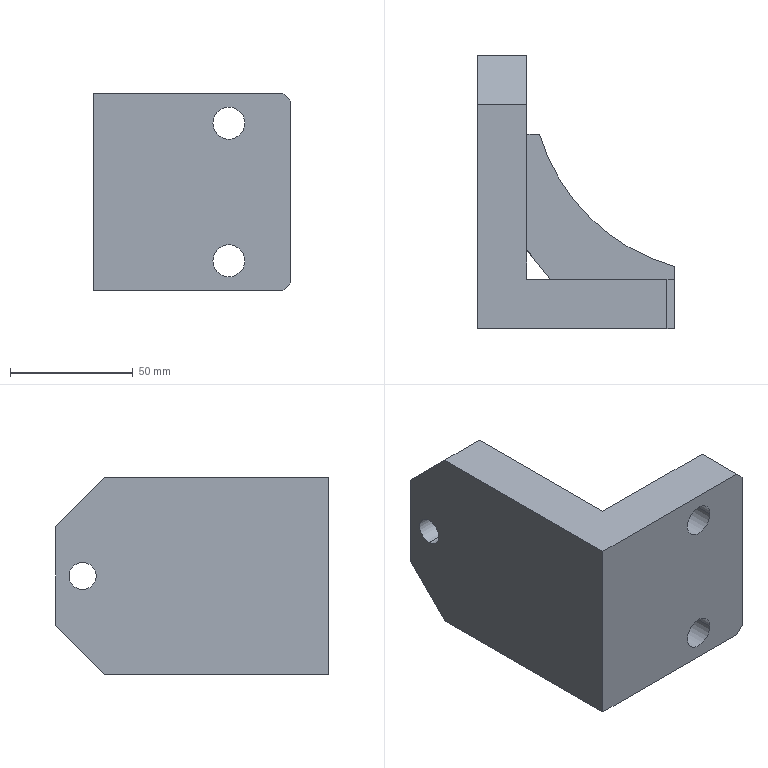Part | Creo | features CURVE 4, DATUM PLANE 3, CHAMFER 2, CUT 2, PROTRUSION 2, COORDINATE SYSTEM 1 | 1 solid | 23 faces | box 80 x 111 x 80 mm | volume 282107 mm3 | plane 16 | cylinder 7 | commonest cylinder face diameters 13 x4 11 x2 158.9 x1
STEP:
#1=CARTESIAN_POINT('',(0.,0.,0.));
#2=DIRECTION('',(0.,0.,1.));
#3=DIRECTION('',(1.,0.,0.));
#4=AXIS2_PLACEMENT_3D('',#1,#2,#3);
#5=CARTESIAN_POINT('',(77.,20.,-40.));
#6=VERTEX_POINT('',#5);
#7=CARTESIAN_POINT('',(77.,0.,-40.));
#8=VERTEX_POINT('',#7);
#9=CARTESIAN_POINT('',(77.,20.,-40.));
#10=DIRECTION('',(0.,-1.,0.));
#11=VECTOR('',#10,20.);
#12=LINE('',#9,#11);
#13=EDGE_CURVE('',#6,#8,#12,.T.);
#14=ORIENTED_EDGE('',*,*,#13,.F.);
#15=CARTESIAN_POINT('',(20.,20.,-40.));
#16=VERTEX_POINT('',#15);
#17=CARTESIAN_POINT('',(77.,20.,-40.));
#18=DIRECTION('',(-1.,0.,0.));
#19=VECTOR('',#18,57.);
#20=LINE('',#17,#19);
#21=EDGE_CURVE('',#6,#16,#20,.T.);
#22=ORIENTED_EDGE('',*,*,#21,.T.);
#23=CARTESIAN_POINT('',(20.,91.,-40.));
#24=VERTEX_POINT('',#23);
#25=CARTESIAN_POINT('',(20.,20.,-40.));
#26=DIRECTION('',(0.,1.,0.));
#27=VECTOR('',#26,71.);
#28=LINE('',#25,#27);
#29=EDGE_CURVE('',#16,#24,#28,.T.);
#30=ORIENTED_EDGE('',*,*,#29,.T.);
#31=CARTESIAN_POINT('',(0.,91.,-40.));
#32=VERTEX_POINT('',#31);
#33=CARTESIAN_POINT('',(0.,91.,-40.));
#34=DIRECTION('',(1.,0.,0.));
#35=VECTOR('',#34,20.);
#36=LINE('',#33,#35);
#37=EDGE_CURVE('',#32,#24,#36,.T.);
#38=ORIENTED_EDGE('',*,*,#37,.F.);
#39=CARTESIAN_POINT('',(0.,0.,-40.));
#40=VERTEX_POINT('',#39);
#41=CARTESIAN_POINT('',(0.,91.,-40.));
#42=DIRECTION('',(0.,-1.,0.));
#43=VECTOR('',#42,91.);
#44=LINE('',#41,#43);
#45=EDGE_CURVE('',#32,#40,#44,.T.);
#46=ORIENTED_EDGE('',*,*,#45,.T.);
#47=CARTESIAN_POINT('',(0.,0.,-40.));
#48=DIRECTION('',(1.,0.,0.));
#49=VECTOR('',#48,77.);
#50=LINE('',#47,#49);
#51=EDGE_CURVE('',#40,#8,#50,.T.);
#52=ORIENTED_EDGE('',*,*,#51,.T.);
#53=EDGE_LOOP('',(#14,#22,#30,#38,#46,#52));
#54=FACE_OUTER_BOUND('',#53,.F.);
#55=CARTESIAN_POINT('',(0.,0.,-40.));
#56=DIRECTION('',(0.,0.,1.));
#57=DIRECTION('',(1.,0.,0.));
#58=AXIS2_PLACEMENT_3D('',#55,#56,#57);
#59=PLANE('',#58);
#60=ADVANCED_FACE('',(#54),#59,.F.);
#61=CARTESIAN_POINT('',(80.,0.,-37.));
#62=VERTEX_POINT('',#61);
#63=CARTESIAN_POINT('',(77.,0.,-40.));
#64=DIRECTION('',(0.7071,0.,0.7071));
#65=VECTOR('',#64,4.243);
#66=LINE('',#63,#65);
#67=EDGE_CURVE('',#8,#62,#66,.T.);
#68=ORIENTED_EDGE('',*,*,#67,.T.);
#69=CARTESIAN_POINT('',(80.,20.,-37.));
#70=VERTEX_POINT('',#69);
#71=CARTESIAN_POINT('',(80.,20.,-37.));
#72=DIRECTION('',(0.,-1.,0.));
#73=VECTOR('',#72,20.);
#74=LINE('',#71,#73);
#75=EDGE_CURVE('',#70,#62,#74,.T.);
#76=ORIENTED_EDGE('',*,*,#75,.F.);
#77=CARTESIAN_POINT('',(80.,20.,-37.));
#78=DIRECTION('',(-0.7071,0.,-0.7071));
#79=VECTOR('',#78,4.243);
#80=LINE('',#77,#79);
#81=EDGE_CURVE('',#70,#6,#80,.T.);
#82=ORIENTED_EDGE('',*,*,#81,.T.);
#83=ORIENTED_EDGE('',*,*,#13,.T.);
#84=EDGE_LOOP('',(#68,#76,#82,#83));
#85=FACE_OUTER_BOUND('',#84,.F.);
#86=CARTESIAN_POINT('',(78.5,10.,-38.5));
#87=DIRECTION('',(0.7071,0.,-0.7071));
#88=DIRECTION('',(0.7071,0.,0.7071));
#89=AXIS2_PLACEMENT_3D('',#86,#87,#88);
#90=PLANE('',#89);
#91=ADVANCED_FACE('',(#85),#90,.T.);
#92=CARTESIAN_POINT('',(80.,0.,37.));
#93=VERTEX_POINT('',#92);
#94=CARTESIAN_POINT('',(77.,0.,40.));
#95=VERTEX_POINT('',#94);
#96=CARTESIAN_POINT('',(80.,0.,37.));
#97=DIRECTION('',(-0.7071,0.,0.7071));
#98=VECTOR('',#97,4.243);
#99=LINE('',#96,#98);
#100=EDGE_CURVE('',#93,#95,#99,.T.);
#101=ORIENTED_EDGE('',*,*,#100,.F.);
#102=CARTESIAN_POINT('',(80.,0.,-37.));
#103=DIRECTION('',(0.,0.,1.));
#104=VECTOR('',#103,74.);
#105=LINE('',#102,#104);
#106=EDGE_CURVE('',#62,#93,#105,.T.);
#107=ORIENTED_EDGE('',*,*,#106,.F.);
#108=ORIENTED_EDGE('',*,*,#67,.F.);
#109=ORIENTED_EDGE('',*,*,#51,.F.);
#110=CARTESIAN_POINT('',(0.,0.,40.));
#111=VERTEX_POINT('',#110);
#112=CARTESIAN_POINT('',(0.,0.,-40.));
#113=DIRECTION('',(0.,0.,1.));
#114=VECTOR('',#113,80.);
#115=LINE('',#112,#114);
#116=EDGE_CURVE('',#40,#111,#115,.T.);
#117=ORIENTED_EDGE('',*,*,#116,.T.);
#118=CARTESIAN_POINT('',(0.,0.,40.));
#119=DIRECTION('',(1.,0.,0.));
#120=VECTOR('',#119,77.);
#121=LINE('',#118,#120);
#122=EDGE_CURVE('',#111,#95,#121,.T.);
#123=ORIENTED_EDGE('',*,*,#122,.T.);
#124=EDGE_LOOP('',(#101,#107,#108,#109,#117,#123));
#125=FACE_OUTER_BOUND('',#124,.F.);
#126=CARTESIAN_POINT('',(61.5,0.,28.));
#127=VERTEX_POINT('',#126);
#128=CARTESIAN_POINT('',(48.5,0.,28.));
#129=VERTEX_POINT('',#128);
#130=CARTESIAN_POINT('',(55.,0.,28.));
#131=DIRECTION('',(0.,1.,0.));
#132=DIRECTION('',(1.,0.,0.));
#133=AXIS2_PLACEMENT_3D('',#130,#131,#132);
#134=CIRCLE('',#133,6.5);
#135=EDGE_CURVE('',#127,#129,#134,.T.);
#136=ORIENTED_EDGE('',*,*,#135,.F.);
#137=CARTESIAN_POINT('',(55.,0.,28.));
#138=DIRECTION('',(0.,1.,0.));
#139=DIRECTION('',(-1.,0.,0.));
#140=AXIS2_PLACEMENT_3D('',#137,#138,#139);
#141=CIRCLE('',#140,6.5);
#142=EDGE_CURVE('',#129,#127,#141,.T.);
#143=ORIENTED_EDGE('',*,*,#142,.F.);
#144=EDGE_LOOP('',(#136,#143));
#145=FACE_BOUND('',#144,.F.);
#146=CARTESIAN_POINT('',(61.5,0.,-28.));
#147=VERTEX_POINT('',#146);
#148=CARTESIAN_POINT('',(48.5,0.,-28.));
#149=VERTEX_POINT('',#148);
#150=CARTESIAN_POINT('',(55.,0.,-28.));
#151=DIRECTION('',(0.,1.,0.));
#152=DIRECTION('',(1.,0.,0.));
#153=AXIS2_PLACEMENT_3D('',#150,#151,#152);
#154=CIRCLE('',#153,6.5);
#155=EDGE_CURVE('',#147,#149,#154,.T.);
#156=ORIENTED_EDGE('',*,*,#155,.F.);
#157=CARTESIAN_POINT('',(55.,0.,-28.));
#158=DIRECTION('',(0.,1.,0.));
#159=DIRECTION('',(-1.,0.,0.));
#160=AXIS2_PLACEMENT_3D('',#157,#158,#159);
#161=CIRCLE('',#160,6.5);
#162=EDGE_CURVE('',#149,#147,#161,.T.);
#163=ORIENTED_EDGE('',*,*,#162,.F.);
#164=EDGE_LOOP('',(#156,#163));
#165=FACE_BOUND('',#164,.F.);
#166=CARTESIAN_POINT('',(0.,0.,-40.));
#167=DIRECTION('',(0.,-1.,0.));
#168=DIRECTION('',(1.,0.,0.));
#169=AXIS2_PLACEMENT_3D('',#166,#167,#168);
#170=PLANE('',#169);
#171=ADVANCED_FACE('',(#125,#145,#165),#170,.T.);
#172=ORIENTED_EDGE('',*,*,#155,.T.);
#173=CARTESIAN_POINT('',(48.5,20.,-28.));
#174=VERTEX_POINT('',#173);
#175=CARTESIAN_POINT('',(48.5,20.,-28.));
#176=DIRECTION('',(0.,-1.,0.));
#177=VECTOR('',#176,20.);
#178=LINE('',#175,#177);
#179=EDGE_CURVE('',#174,#149,#178,.T.);
#180=ORIENTED_EDGE('',*,*,#179,.F.);
#181=CARTESIAN_POINT('',(61.5,20.,-28.));
#182=VERTEX_POINT('',#181);
#183=CARTESIAN_POINT('',(55.,20.,-28.));
#184=DIRECTION('',(0.,1.,0.));
#185=DIRECTION('',(1.,0.,0.));
#186=AXIS2_PLACEMENT_3D('',#183,#184,#185);
#187=CIRCLE('',#186,6.5);
#188=EDGE_CURVE('',#182,#174,#187,.T.);
#189=ORIENTED_EDGE('',*,*,#188,.F.);
#190=CARTESIAN_POINT('',(61.5,20.,-28.));
#191=DIRECTION('',(0.,-1.,0.));
#192=VECTOR('',#191,20.);
#193=LINE('',#190,#192);
#194=EDGE_CURVE('',#182,#147,#193,.T.);
#195=ORIENTED_EDGE('',*,*,#194,.T.);
#196=EDGE_LOOP('',(#172,#180,#189,#195));
#197=FACE_OUTER_BOUND('',#196,.F.);
#198=CARTESIAN_POINT('',(55.,20.,-28.));
#199=DIRECTION('',(0.,1.,0.));
#200=DIRECTION('',(1.,0.,0.));
#201=AXIS2_PLACEMENT_3D('',#198,#199,#200);
#202=CYLINDRICAL_SURFACE('',#201,6.5);
#203=ADVANCED_FACE('',(#197),#202,.F.);
#204=ORIENTED_EDGE('',*,*,#162,.T.);
#205=ORIENTED_EDGE('',*,*,#194,.F.);
#206=CARTESIAN_POINT('',(55.,20.,-28.));
#207=DIRECTION('',(0.,1.,0.));
#208=DIRECTION('',(-1.,0.,0.));
#209=AXIS2_PLACEMENT_3D('',#206,#207,#208);
#210=CIRCLE('',#209,6.5);
#211=EDGE_CURVE('',#174,#182,#210,.T.);
#212=ORIENTED_EDGE('',*,*,#211,.F.);
#213=ORIENTED_EDGE('',*,*,#179,.T.);
#214=EDGE_LOOP('',(#204,#205,#212,#213));
#215=FACE_OUTER_BOUND('',#214,.F.);
#216=CARTESIAN_POINT('',(55.,20.,-28.));
#217=DIRECTION('',(0.,1.,0.));
#218=DIRECTION('',(1.,0.,0.));
#219=AXIS2_PLACEMENT_3D('',#216,#217,#218);
#220=CYLINDRICAL_SURFACE('',#219,6.5);
#221=ADVANCED_FACE('',(#215),#220,.F.);
#222=CARTESIAN_POINT('',(77.,20.,40.));
#223=VERTEX_POINT('',#222);
#224=CARTESIAN_POINT('',(80.,20.,37.));
#225=VERTEX_POINT('',#224);
#226=CARTESIAN_POINT('',(77.,20.,40.));
#227=DIRECTION('',(0.7071,0.,-0.7071));
#228=VECTOR('',#227,4.243);
#229=LINE('',#226,#228);
#230=EDGE_CURVE('',#223,#225,#229,.T.);
#231=ORIENTED_EDGE('',*,*,#230,.F.);
#232=CARTESIAN_POINT('',(20.,20.,40.));
#233=VERTEX_POINT('',#232);
#234=CARTESIAN_POINT('',(77.,20.,40.));
#235=DIRECTION('',(-1.,0.,0.));
#236=VECTOR('',#235,57.);
#237=LINE('',#234,#236);
#238=EDGE_CURVE('',#223,#233,#237,.T.);
#239=ORIENTED_EDGE('',*,*,#238,.T.);
#240=CARTESIAN_POINT('',(20.,20.,-40.));
#241=DIRECTION('',(0.,0.,1.));
#242=VECTOR('',#241,80.);
#243=LINE('',#240,#242);
#244=EDGE_CURVE('',#16,#233,#243,.T.);
#245=ORIENTED_EDGE('',*,*,#244,.F.);
#246=ORIENTED_EDGE('',*,*,#21,.F.);
#247=ORIENTED_EDGE('',*,*,#81,.F.);
#248=CARTESIAN_POINT('',(80.,20.,-8.));
#249=VERTEX_POINT('',#248);
#250=CARTESIAN_POINT('',(80.,20.,-37.));
#251=DIRECTION('',(0.,0.,1.));
#252=VECTOR('',#251,29.);
#253=LINE('',#250,#252);
#254=EDGE_CURVE('',#70,#249,#253,.T.);
#255=ORIENTED_EDGE('',*,*,#254,.T.);
#256=CARTESIAN_POINT('',(29.611,20.,-8.));
#257=VERTEX_POINT('',#256);
#258=CARTESIAN_POINT('',(80.,20.,-8.));
#259=DIRECTION('',(-1.,0.,0.));
#260=VECTOR('',#259,50.389);
#261=LINE('',#258,#260);
#262=EDGE_CURVE('',#249,#257,#261,.T.);
#263=ORIENTED_EDGE('',*,*,#262,.T.);
#264=CARTESIAN_POINT('',(29.611,20.,8.));
#265=VERTEX_POINT('',#264);
#266=CARTESIAN_POINT('',(29.611,20.,-8.));
#267=DIRECTION('',(0.,0.,1.));
#268=VECTOR('',#267,16.);
#269=LINE('',#266,#268);
#270=EDGE_CURVE('',#257,#265,#269,.T.);
#271=ORIENTED_EDGE('',*,*,#270,.T.);
#272=CARTESIAN_POINT('',(80.,20.,8.));
#273=VERTEX_POINT('',#272);
#274=CARTESIAN_POINT('',(80.,20.,8.));
#275=DIRECTION('',(-1.,0.,0.));
#276=VECTOR('',#275,50.389);
#277=LINE('',#274,#276);
#278=EDGE_CURVE('',#273,#265,#277,.T.);
#279=ORIENTED_EDGE('',*,*,#278,.F.);
#280=CARTESIAN_POINT('',(80.,20.,8.));
#281=DIRECTION('',(0.,0.,1.));
#282=VECTOR('',#281,29.);
#283=LINE('',#280,#282);
#284=EDGE_CURVE('',#273,#225,#283,.T.);
#285=ORIENTED_EDGE('',*,*,#284,.T.);
#286=EDGE_LOOP('',(#231,#239,#245,#246,#247,#255,#263,#271,#279,#285));
#287=FACE_OUTER_BOUND('',#286,.F.);
#288=CARTESIAN_POINT('',(61.5,20.,28.));
#289=VERTEX_POINT('',#288);
#290=CARTESIAN_POINT('',(48.5,20.,28.));
#291=VERTEX_POINT('',#290);
#292=CARTESIAN_POINT('',(55.,20.,28.));
#293=DIRECTION('',(0.,1.,0.));
#294=DIRECTION('',(1.,0.,0.));
#295=AXIS2_PLACEMENT_3D('',#292,#293,#294);
#296=CIRCLE('',#295,6.5);
#297=EDGE_CURVE('',#289,#291,#296,.T.);
#298=ORIENTED_EDGE('',*,*,#297,.T.);
#299=CARTESIAN_POINT('',(55.,20.,28.));
#300=DIRECTION('',(0.,1.,0.));
#301=DIRECTION('',(-1.,0.,0.));
#302=AXIS2_PLACEMENT_3D('',#299,#300,#301);
#303=CIRCLE('',#302,6.5);
#304=EDGE_CURVE('',#291,#289,#303,.T.);
#305=ORIENTED_EDGE('',*,*,#304,.T.);
#306=EDGE_LOOP('',(#298,#305));
#307=FACE_BOUND('',#306,.F.);
#308=ORIENTED_EDGE('',*,*,#188,.T.);
#309=ORIENTED_EDGE('',*,*,#211,.T.);
#310=EDGE_LOOP('',(#308,#309));
#311=FACE_BOUND('',#310,.F.);
#312=CARTESIAN_POINT('',(80.,20.,-40.));
#313=DIRECTION('',(0.,1.,0.));
#314=DIRECTION('',(-1.,0.,0.));
#315=AXIS2_PLACEMENT_3D('',#312,#313,#314);
#316=PLANE('',#315);
#317=ADVANCED_FACE('',(#287,#307,#311),#316,.T.);
#318=ORIENTED_EDGE('',*,*,#135,.T.);
#319=CARTESIAN_POINT('',(48.5,20.,28.));
#320=DIRECTION('',(0.,-1.,0.));
#321=VECTOR('',#320,20.);
#322=LINE('',#319,#321);
#323=EDGE_CURVE('',#291,#129,#322,.T.);
#324=ORIENTED_EDGE('',*,*,#323,.F.);
#325=ORIENTED_EDGE('',*,*,#297,.F.);
#326=CARTESIAN_POINT('',(61.5,20.,28.));
#327=DIRECTION('',(0.,-1.,0.));
#328=VECTOR('',#327,20.);
#329=LINE('',#326,#328);
#330=EDGE_CURVE('',#289,#127,#329,.T.);
#331=ORIENTED_EDGE('',*,*,#330,.T.);
#332=EDGE_LOOP('',(#318,#324,#325,#331));
#333=FACE_OUTER_BOUND('',#332,.F.);
#334=CARTESIAN_POINT('',(55.,20.,28.));
#335=DIRECTION('',(0.,1.,0.));
#336=DIRECTION('',(1.,0.,0.));
#337=AXIS2_PLACEMENT_3D('',#334,#335,#336);
#338=CYLINDRICAL_SURFACE('',#337,6.5);
#339=ADVANCED_FACE('',(#333),#338,.F.);
#340=ORIENTED_EDGE('',*,*,#142,.T.);
#341=ORIENTED_EDGE('',*,*,#330,.F.);
#342=ORIENTED_EDGE('',*,*,#304,.F.);
#343=ORIENTED_EDGE('',*,*,#323,.T.);
#344=EDGE_LOOP('',(#340,#341,#342,#343));
#345=FACE_OUTER_BOUND('',#344,.F.);
#346=CARTESIAN_POINT('',(55.,20.,28.));
#347=DIRECTION('',(0.,1.,0.));
#348=DIRECTION('',(1.,0.,0.));
#349=AXIS2_PLACEMENT_3D('',#346,#347,#348);
#350=CYLINDRICAL_SURFACE('',#349,6.5);
#351=ADVANCED_FACE('',(#345),#350,.F.);
#352=ORIENTED_EDGE('',*,*,#230,.T.);
#353=CARTESIAN_POINT('',(80.,0.,37.));
#354=DIRECTION('',(0.,1.,0.));
#355=VECTOR('',#354,20.);
#356=LINE('',#353,#355);
#357=EDGE_CURVE('',#93,#225,#356,.T.);
#358=ORIENTED_EDGE('',*,*,#357,.F.);
#359=ORIENTED_EDGE('',*,*,#100,.T.);
#360=CARTESIAN_POINT('',(77.,0.,40.));
#361=DIRECTION('',(0.,1.,0.));
#362=VECTOR('',#361,20.);
#363=LINE('',#360,#362);
#364=EDGE_CURVE('',#95,#223,#363,.T.);
#365=ORIENTED_EDGE('',*,*,#364,.T.);
#366=EDGE_LOOP('',(#352,#358,#359,#365));
#367=FACE_OUTER_BOUND('',#366,.F.);
#368=CARTESIAN_POINT('',(78.5,10.,38.5));
#369=DIRECTION('',(0.7071,0.,0.7071));
#370=DIRECTION('',(0.7071,0.,-0.7071));
#371=AXIS2_PLACEMENT_3D('',#368,#369,#370);
#372=PLANE('',#371);
#373=ADVANCED_FACE('',(#367),#372,.T.);
#374=ORIENTED_EDGE('',*,*,#357,.T.);
#375=ORIENTED_EDGE('',*,*,#284,.F.);
#376=CARTESIAN_POINT('',(80.,25.177,8.));
#377=VERTEX_POINT('',#376);
#378=CARTESIAN_POINT('',(80.,20.,8.));
#379=DIRECTION('',(0.,1.,0.));
#380=VECTOR('',#379,5.177);
#381=LINE('',#378,#380);
#382=EDGE_CURVE('',#273,#377,#381,.T.);
#383=ORIENTED_EDGE('',*,*,#382,.T.);
#384=CARTESIAN_POINT('',(80.,25.177,-8.));
#385=VERTEX_POINT('',#384);
#386=CARTESIAN_POINT('',(80.,25.177,-8.));
#387=DIRECTION('',(0.,0.,1.));
#388=VECTOR('',#387,16.);
#389=LINE('',#386,#388);
#390=EDGE_CURVE('',#385,#377,#389,.T.);
#391=ORIENTED_EDGE('',*,*,#390,.F.);
#392=CARTESIAN_POINT('',(80.,20.,-8.));
#393=DIRECTION('',(0.,1.,0.));
#394=VECTOR('',#393,5.177);
#395=LINE('',#392,#394);
#396=EDGE_CURVE('',#249,#385,#395,.T.);
#397=ORIENTED_EDGE('',*,*,#396,.F.);
#398=ORIENTED_EDGE('',*,*,#254,.F.);
#399=ORIENTED_EDGE('',*,*,#75,.T.);
#400=ORIENTED_EDGE('',*,*,#106,.T.);
#401=EDGE_LOOP('',(#374,#375,#383,#391,#397,#398,#399,#400));
#402=FACE_OUTER_BOUND('',#401,.F.);
#403=CARTESIAN_POINT('',(80.,0.,-40.));
#404=DIRECTION('',(1.,0.,0.));
#405=DIRECTION('',(0.,1.,0.));
#406=AXIS2_PLACEMENT_3D('',#403,#404,#405);
#407=PLANE('',#406);
#408=ADVANCED_FACE('',(#402),#407,.T.);
#409=ORIENTED_EDGE('',*,*,#278,.T.);
#410=CARTESIAN_POINT('',(20.,31.895,8.));
#411=VERTEX_POINT('',#410);
#412=CARTESIAN_POINT('',(20.,31.895,8.));
#413=DIRECTION('',(0.6285,-0.7778,0.));
#414=VECTOR('',#413,15.293);
#415=LINE('',#412,#414);
#416=EDGE_CURVE('',#411,#265,#415,.T.);
#417=ORIENTED_EDGE('',*,*,#416,.F.);
#418=CARTESIAN_POINT('',(20.,79.,8.));
#419=VERTEX_POINT('',#418);
#420=CARTESIAN_POINT('',(20.,31.895,8.));
#421=DIRECTION('',(0.,1.,0.));
#422=VECTOR('',#421,47.105);
#423=LINE('',#420,#422);
#424=EDGE_CURVE('',#411,#419,#423,.T.);
#425=ORIENTED_EDGE('',*,*,#424,.T.);
#426=CARTESIAN_POINT('',(25.177,79.,8.));
#427=VERTEX_POINT('',#426);
#428=CARTESIAN_POINT('',(25.177,79.,8.));
#429=DIRECTION('',(-1.,0.,0.));
#430=VECTOR('',#429,5.177);
#431=LINE('',#428,#430);
#432=EDGE_CURVE('',#427,#419,#431,.T.);
#433=ORIENTED_EDGE('',*,*,#432,.F.);
#434=CARTESIAN_POINT('',(101.311,101.716,8.));
#435=DIRECTION('',(0.,0.,-1.));
#436=DIRECTION('',(-0.2682,-0.9634,0.));
#437=AXIS2_PLACEMENT_3D('',#434,#435,#436);
#438=CIRCLE('',#437,79.45);
#439=EDGE_CURVE('',#377,#427,#438,.T.);
#440=ORIENTED_EDGE('',*,*,#439,.F.);
#441=ORIENTED_EDGE('',*,*,#382,.F.);
#442=EDGE_LOOP('',(#409,#417,#425,#433,#440,#441));
#443=FACE_OUTER_BOUND('',#442,.F.);
#444=CARTESIAN_POINT('',(0.,0.,8.));
#445=DIRECTION('',(0.,0.,1.));
#446=DIRECTION('',(1.,0.,0.));
#447=AXIS2_PLACEMENT_3D('',#444,#445,#446);
#448=PLANE('',#447);
#449=ADVANCED_FACE('',(#443),#448,.T.);
#450=ORIENTED_EDGE('',*,*,#270,.F.);
#451=CARTESIAN_POINT('',(20.,31.895,-8.));
#452=VERTEX_POINT('',#451);
#453=CARTESIAN_POINT('',(20.,31.895,-8.));
#454=DIRECTION('',(0.6285,-0.7778,0.));
#455=VECTOR('',#454,15.293);
#456=LINE('',#453,#455);
#457=EDGE_CURVE('',#452,#257,#456,.T.);
#458=ORIENTED_EDGE('',*,*,#457,.F.);
#459=CARTESIAN_POINT('',(20.,31.895,-8.));
#460=DIRECTION('',(0.,0.,1.));
#461=VECTOR('',#460,16.);
#462=LINE('',#459,#461);
#463=EDGE_CURVE('',#452,#411,#462,.T.);
#464=ORIENTED_EDGE('',*,*,#463,.T.);
#465=ORIENTED_EDGE('',*,*,#416,.T.);
#466=EDGE_LOOP('',(#450,#458,#464,#465));
#467=FACE_OUTER_BOUND('',#466,.F.);
#468=CARTESIAN_POINT('',(20.,31.895,-8.));
#469=DIRECTION('',(-0.7778,-0.6285,0.));
#470=DIRECTION('',(0.6285,-0.7778,0.));
#471=AXIS2_PLACEMENT_3D('',#468,#469,#470);
#472=PLANE('',#471);
#473=ADVANCED_FACE('',(#467),#472,.T.);
#474=ORIENTED_EDGE('',*,*,#262,.F.);
#475=ORIENTED_EDGE('',*,*,#396,.T.);
#476=CARTESIAN_POINT('',(25.177,79.,-8.));
#477=VERTEX_POINT('',#476);
#478=CARTESIAN_POINT('',(101.311,101.716,-8.));
#479=DIRECTION('',(0.,0.,-1.));
#480=DIRECTION('',(-0.2682,-0.9634,0.));
#481=AXIS2_PLACEMENT_3D('',#478,#479,#480);
#482=CIRCLE('',#481,79.45);
#483=EDGE_CURVE('',#385,#477,#482,.T.);
#484=ORIENTED_EDGE('',*,*,#483,.T.);
#485=CARTESIAN_POINT('',(20.,79.,-8.));
#486=VERTEX_POINT('',#485);
#487=CARTESIAN_POINT('',(25.177,79.,-8.));
#488=DIRECTION('',(-1.,0.,0.));
#489=VECTOR('',#488,5.177);
#490=LINE('',#487,#489);
#491=EDGE_CURVE('',#477,#486,#490,.T.);
#492=ORIENTED_EDGE('',*,*,#491,.T.);
#493=CARTESIAN_POINT('',(20.,31.895,-8.));
#494=DIRECTION('',(0.,1.,0.));
#495=VECTOR('',#494,47.105);
#496=LINE('',#493,#495);
#497=EDGE_CURVE('',#452,#486,#496,.T.);
#498=ORIENTED_EDGE('',*,*,#497,.F.);
#499=ORIENTED_EDGE('',*,*,#457,.T.);
#500=EDGE_LOOP('',(#474,#475,#484,#492,#498,#499));
#501=FACE_OUTER_BOUND('',#500,.F.);
#502=CARTESIAN_POINT('',(0.,0.,-8.));
#503=DIRECTION('',(0.,0.,1.));
#504=DIRECTION('',(1.,0.,0.));
#505=AXIS2_PLACEMENT_3D('',#502,#503,#504);
#506=PLANE('',#505);
#507=ADVANCED_FACE('',(#501),#506,.F.);
#508=ORIENTED_EDGE('',*,*,#483,.F.);
#509=ORIENTED_EDGE('',*,*,#390,.T.);
#510=ORIENTED_EDGE('',*,*,#439,.T.);
#511=CARTESIAN_POINT('',(25.177,79.,-8.));
#512=DIRECTION('',(0.,0.,1.));
#513=VECTOR('',#512,16.);
#514=LINE('',#511,#513);
#515=EDGE_CURVE('',#477,#427,#514,.T.);
#516=ORIENTED_EDGE('',*,*,#515,.F.);
#517=EDGE_LOOP('',(#508,#509,#510,#516));
#518=FACE_OUTER_BOUND('',#517,.F.);
#519=CARTESIAN_POINT('',(101.311,101.716,-8.));
#520=DIRECTION('',(0.,0.,1.));
#521=DIRECTION('',(1.,0.,0.));
#522=AXIS2_PLACEMENT_3D('',#519,#520,#521);
#523=CYLINDRICAL_SURFACE('',#522,79.45);
#524=ADVANCED_FACE('',(#518),#523,.F.);
#525=CARTESIAN_POINT('',(20.,79.,-8.));
#526=DIRECTION('',(0.,0.,1.));
#527=VECTOR('',#526,16.);
#528=LINE('',#525,#527);
#529=EDGE_CURVE('',#486,#419,#528,.T.);
#530=ORIENTED_EDGE('',*,*,#529,.F.);
#531=ORIENTED_EDGE('',*,*,#491,.F.);
#532=ORIENTED_EDGE('',*,*,#515,.T.);
#533=ORIENTED_EDGE('',*,*,#432,.T.);
#534=EDGE_LOOP('',(#530,#531,#532,#533));
#535=FACE_OUTER_BOUND('',#534,.F.);
#536=CARTESIAN_POINT('',(25.177,79.,-8.));
#537=DIRECTION('',(0.,1.,0.));
#538=DIRECTION('',(-1.,0.,0.));
#539=AXIS2_PLACEMENT_3D('',#536,#537,#538);
#540=PLANE('',#539);
#541=ADVANCED_FACE('',(#535),#540,.T.);
#542=CARTESIAN_POINT('',(20.,111.,20.));
#543=VERTEX_POINT('',#542);
#544=CARTESIAN_POINT('',(20.,91.,40.));
#545=VERTEX_POINT('',#544);
#546=CARTESIAN_POINT('',(20.,111.,20.));
#547=DIRECTION('',(0.,-0.7071,0.7071));
#548=VECTOR('',#547,28.284);
#549=LINE('',#546,#548);
#550=EDGE_CURVE('',#543,#545,#549,.T.);
#551=ORIENTED_EDGE('',*,*,#550,.F.);
#552=CARTESIAN_POINT('',(20.,111.,-20.));
#553=VERTEX_POINT('',#552);
#554=CARTESIAN_POINT('',(20.,111.,-20.));
#555=DIRECTION('',(0.,0.,1.));
#556=VECTOR('',#555,40.);
#557=LINE('',#554,#556);
#558=EDGE_CURVE('',#553,#543,#557,.T.);
#559=ORIENTED_EDGE('',*,*,#558,.F.);
#560=CARTESIAN_POINT('',(20.,91.,-40.));
#561=DIRECTION('',(0.,0.7071,0.7071));
#562=VECTOR('',#561,28.284);
#563=LINE('',#560,#562);
#564=EDGE_CURVE('',#24,#553,#563,.T.);
#565=ORIENTED_EDGE('',*,*,#564,.F.);
#566=ORIENTED_EDGE('',*,*,#29,.F.);
#567=ORIENTED_EDGE('',*,*,#244,.T.);
#568=CARTESIAN_POINT('',(20.,20.,40.));
#569=DIRECTION('',(0.,1.,0.));
#570=VECTOR('',#569,71.);
#571=LINE('',#568,#570);
#572=EDGE_CURVE('',#233,#545,#571,.T.);
#573=ORIENTED_EDGE('',*,*,#572,.T.);
#574=EDGE_LOOP('',(#551,#559,#565,#566,#567,#573));
#575=FACE_OUTER_BOUND('',#574,.F.);
#576=CARTESIAN_POINT('',(20.,100.,-5.5));
#577=VERTEX_POINT('',#576);
#578=CARTESIAN_POINT('',(20.,100.,5.5));
#579=VERTEX_POINT('',#578);
#580=CARTESIAN_POINT('',(20.,100.,0.));
#581=DIRECTION('',(1.,0.,0.));
#582=DIRECTION('',(0.,0.,-1.));
#583=AXIS2_PLACEMENT_3D('',#580,#581,#582);
#584=CIRCLE('',#583,5.5);
#585=EDGE_CURVE('',#577,#579,#584,.T.);
#586=ORIENTED_EDGE('',*,*,#585,.T.);
#587=CARTESIAN_POINT('',(20.,100.,0.));
#588=DIRECTION('',(1.,0.,0.));
#589=DIRECTION('',(0.,0.,1.));
#590=AXIS2_PLACEMENT_3D('',#587,#588,#589);
#591=CIRCLE('',#590,5.5);
#592=EDGE_CURVE('',#579,#577,#591,.T.);
#593=ORIENTED_EDGE('',*,*,#592,.T.);
#594=EDGE_LOOP('',(#586,#593));
#595=FACE_BOUND('',#594,.F.);
#596=ORIENTED_EDGE('',*,*,#497,.T.);
#597=ORIENTED_EDGE('',*,*,#529,.T.);
#598=ORIENTED_EDGE('',*,*,#424,.F.);
#599=ORIENTED_EDGE('',*,*,#463,.F.);
#600=EDGE_LOOP('',(#596,#597,#598,#599));
#601=FACE_BOUND('',#600,.F.);
#602=CARTESIAN_POINT('',(20.,20.,-40.));
#603=DIRECTION('',(1.,0.,0.));
#604=DIRECTION('',(0.,1.,0.));
#605=AXIS2_PLACEMENT_3D('',#602,#603,#604);
#606=PLANE('',#605);
#607=ADVANCED_FACE('',(#575,#595,#601),#606,.T.);
#608=CARTESIAN_POINT('',(0.,100.,-5.5));
#609=VERTEX_POINT('',#608);
#610=CARTESIAN_POINT('',(0.,100.,5.5));
#611=VERTEX_POINT('',#610);
#612=CARTESIAN_POINT('',(0.,100.,0.));
#613=DIRECTION('',(1.,0.,0.));
#614=DIRECTION('',(0.,0.,-1.));
#615=AXIS2_PLACEMENT_3D('',#612,#613,#614);
#616=CIRCLE('',#615,5.5);
#617=EDGE_CURVE('',#609,#611,#616,.T.);
#618=ORIENTED_EDGE('',*,*,#617,.T.);
#619=CARTESIAN_POINT('',(20.,100.,5.5));
#620=DIRECTION('',(-1.,0.,0.));
#621=VECTOR('',#620,20.);
#622=LINE('',#619,#621);
#623=EDGE_CURVE('',#579,#611,#622,.T.);
#624=ORIENTED_EDGE('',*,*,#623,.F.);
#625=ORIENTED_EDGE('',*,*,#585,.F.);
#626=CARTESIAN_POINT('',(20.,100.,-5.5));
#627=DIRECTION('',(-1.,0.,0.));
#628=VECTOR('',#627,20.);
#629=LINE('',#626,#628);
#630=EDGE_CURVE('',#577,#609,#629,.T.);
#631=ORIENTED_EDGE('',*,*,#630,.T.);
#632=EDGE_LOOP('',(#618,#624,#625,#631));
#633=FACE_OUTER_BOUND('',#632,.F.);
#634=CARTESIAN_POINT('',(20.,100.,0.));
#635=DIRECTION('',(1.,0.,0.));
#636=DIRECTION('',(0.,0.,-1.));
#637=AXIS2_PLACEMENT_3D('',#634,#635,#636);
#638=CYLINDRICAL_SURFACE('',#637,5.5);
#639=ADVANCED_FACE('',(#633),#638,.F.);
#640=CARTESIAN_POINT('',(0.,91.,40.));
#641=VERTEX_POINT('',#640);
#642=CARTESIAN_POINT('',(0.,111.,20.));
#643=VERTEX_POINT('',#642);
#644=CARTESIAN_POINT('',(0.,91.,40.));
#645=DIRECTION('',(0.,0.7071,-0.7071));
#646=VECTOR('',#645,28.284);
#647=LINE('',#644,#646);
#648=EDGE_CURVE('',#641,#643,#647,.T.);
#649=ORIENTED_EDGE('',*,*,#648,.F.);
#650=CARTESIAN_POINT('',(0.,91.,40.));
#651=DIRECTION('',(0.,-1.,0.));
#652=VECTOR('',#651,91.);
#653=LINE('',#650,#652);
#654=EDGE_CURVE('',#641,#111,#653,.T.);
#655=ORIENTED_EDGE('',*,*,#654,.T.);
#656=ORIENTED_EDGE('',*,*,#116,.F.);
#657=ORIENTED_EDGE('',*,*,#45,.F.);
#658=CARTESIAN_POINT('',(0.,111.,-20.));
#659=VERTEX_POINT('',#658);
#660=CARTESIAN_POINT('',(0.,111.,-20.));
#661=DIRECTION('',(0.,-0.7071,-0.7071));
#662=VECTOR('',#661,28.284);
#663=LINE('',#660,#662);
#664=EDGE_CURVE('',#659,#32,#663,.T.);
#665=ORIENTED_EDGE('',*,*,#664,.F.);
#666=CARTESIAN_POINT('',(0.,111.,-20.));
#667=DIRECTION('',(0.,0.,1.));
#668=VECTOR('',#667,40.);
#669=LINE('',#666,#668);
#670=EDGE_CURVE('',#659,#643,#669,.T.);
#671=ORIENTED_EDGE('',*,*,#670,.T.);
#672=EDGE_LOOP('',(#649,#655,#656,#657,#665,#671));
#673=FACE_OUTER_BOUND('',#672,.F.);
#674=ORIENTED_EDGE('',*,*,#617,.F.);
#675=CARTESIAN_POINT('',(0.,100.,0.));
#676=DIRECTION('',(1.,0.,0.));
#677=DIRECTION('',(0.,0.,1.));
#678=AXIS2_PLACEMENT_3D('',#675,#676,#677);
#679=CIRCLE('',#678,5.5);
#680=EDGE_CURVE('',#611,#609,#679,.T.);
#681=ORIENTED_EDGE('',*,*,#680,.F.);
#682=EDGE_LOOP('',(#674,#681));
#683=FACE_BOUND('',#682,.F.);
#684=CARTESIAN_POINT('',(0.,111.,-40.));
#685=DIRECTION('',(-1.,0.,0.));
#686=DIRECTION('',(0.,-1.,0.));
#687=AXIS2_PLACEMENT_3D('',#684,#685,#686);
#688=PLANE('',#687);
#689=ADVANCED_FACE('',(#673,#683),#688,.T.);
#690=ORIENTED_EDGE('',*,*,#680,.T.);
#691=ORIENTED_EDGE('',*,*,#630,.F.);
#692=ORIENTED_EDGE('',*,*,#592,.F.);
#693=ORIENTED_EDGE('',*,*,#623,.T.);
#694=EDGE_LOOP('',(#690,#691,#692,#693));
#695=FACE_OUTER_BOUND('',#694,.F.);
#696=CARTESIAN_POINT('',(20.,100.,0.));
#697=DIRECTION('',(1.,0.,0.));
#698=DIRECTION('',(0.,0.,-1.));
#699=AXIS2_PLACEMENT_3D('',#696,#697,#698);
#700=CYLINDRICAL_SURFACE('',#699,5.5);
#701=ADVANCED_FACE('',(#695),#700,.F.);
#702=ORIENTED_EDGE('',*,*,#648,.T.);
#703=CARTESIAN_POINT('',(20.,111.,20.));
#704=DIRECTION('',(-1.,0.,0.));
#705=VECTOR('',#704,20.);
#706=LINE('',#703,#705);
#707=EDGE_CURVE('',#543,#643,#706,.T.);
#708=ORIENTED_EDGE('',*,*,#707,.F.);
#709=ORIENTED_EDGE('',*,*,#550,.T.);
#710=CARTESIAN_POINT('',(20.,91.,40.));
#711=DIRECTION('',(-1.,0.,0.));
#712=VECTOR('',#711,20.);
#713=LINE('',#710,#712);
#714=EDGE_CURVE('',#545,#641,#713,.T.);
#715=ORIENTED_EDGE('',*,*,#714,.T.);
#716=EDGE_LOOP('',(#702,#708,#709,#715));
#717=FACE_OUTER_BOUND('',#716,.F.);
#718=CARTESIAN_POINT('',(10.,101.,30.));
#719=DIRECTION('',(0.,0.7071,0.7071));
#720=DIRECTION('',(0.,0.7071,-0.7071));
#721=AXIS2_PLACEMENT_3D('',#718,#719,#720);
#722=PLANE('',#721);
#723=ADVANCED_FACE('',(#717),#722,.T.);
#724=ORIENTED_EDGE('',*,*,#707,.T.);
#725=ORIENTED_EDGE('',*,*,#670,.F.);
#726=CARTESIAN_POINT('',(0.,111.,-20.));
#727=DIRECTION('',(1.,0.,0.));
#728=VECTOR('',#727,20.);
#729=LINE('',#726,#728);
#730=EDGE_CURVE('',#659,#553,#729,.T.);
#731=ORIENTED_EDGE('',*,*,#730,.T.);
#732=ORIENTED_EDGE('',*,*,#558,.T.);
#733=EDGE_LOOP('',(#724,#725,#731,#732));
#734=FACE_OUTER_BOUND('',#733,.F.);
#735=CARTESIAN_POINT('',(20.,111.,-40.));
#736=DIRECTION('',(0.,1.,0.));
#737=DIRECTION('',(-1.,0.,0.));
#738=AXIS2_PLACEMENT_3D('',#735,#736,#737);
#739=PLANE('',#738);
#740=ADVANCED_FACE('',(#734),#739,.T.);
#741=ORIENTED_EDGE('',*,*,#564,.T.);
#742=ORIENTED_EDGE('',*,*,#730,.F.);
#743=ORIENTED_EDGE('',*,*,#664,.T.);
#744=ORIENTED_EDGE('',*,*,#37,.T.);
#745=EDGE_LOOP('',(#741,#742,#743,#744));
#746=FACE_OUTER_BOUND('',#745,.F.);
#747=CARTESIAN_POINT('',(10.,101.,-30.));
#748=DIRECTION('',(0.,0.7071,-0.7071));
#749=DIRECTION('',(0.,0.7071,0.7071));
#750=AXIS2_PLACEMENT_3D('',#747,#748,#749);
#751=PLANE('',#750);
#752=ADVANCED_FACE('',(#746),#751,.T.);
#753=ORIENTED_EDGE('',*,*,#364,.F.);
#754=ORIENTED_EDGE('',*,*,#122,.F.);
#755=ORIENTED_EDGE('',*,*,#654,.F.);
#756=ORIENTED_EDGE('',*,*,#714,.F.);
#757=ORIENTED_EDGE('',*,*,#572,.F.);
#758=ORIENTED_EDGE('',*,*,#238,.F.);
#759=EDGE_LOOP('',(#753,#754,#755,#756,#757,#758));
#760=FACE_OUTER_BOUND('',#759,.F.);
#761=CARTESIAN_POINT('',(0.,0.,40.));
#762=DIRECTION('',(0.,0.,1.));
#763=DIRECTION('',(1.,0.,0.));
#764=AXIS2_PLACEMENT_3D('',#761,#762,#763);
#765=PLANE('',#764);
#766=ADVANCED_FACE('',(#760),#765,.T.);
#767=CLOSED_SHELL('',(#60,#91,#171,#203,#221,#317,#339,#351,#373,#408,#449,#473,#507,#524,#541,#607,#639,#689,#701,#723,#740,#752,#766));
#768=MANIFOLD_SOLID_BREP('',#767);
#769=(LENGTH_UNIT()NAMED_UNIT(*)SI_UNIT(.MILLI.,.METRE.));
#770=UNCERTAINTY_MEASURE_WITH_UNIT(LENGTH_MEASURE(0.01585),#769,'','');
#771=(NAMED_UNIT(*)PLANE_ANGLE_UNIT()SI_UNIT($,.RADIAN.));
#772=PLANE_ANGLE_MEASURE_WITH_UNIT(PLANE_ANGLE_MEASURE(0.01745),#771);
#773=(CONVERSION_BASED_UNIT('DEGREE',#772)NAMED_UNIT(*)PLANE_ANGLE_UNIT());
#774=(NAMED_UNIT(*)SI_UNIT($,.STERADIAN.)SOLID_ANGLE_UNIT());
#775=(GEOMETRIC_REPRESENTATION_CONTEXT(3)GLOBAL_UNCERTAINTY_ASSIGNED_CONTEXT((#770))GLOBAL_UNIT_ASSIGNED_CONTEXT((#769,#773,#774))REPRESENTATION_CONTEXT('',''));
#776=ADVANCED_BREP_SHAPE_REPRESENTATION('',(#4,#768),#775);